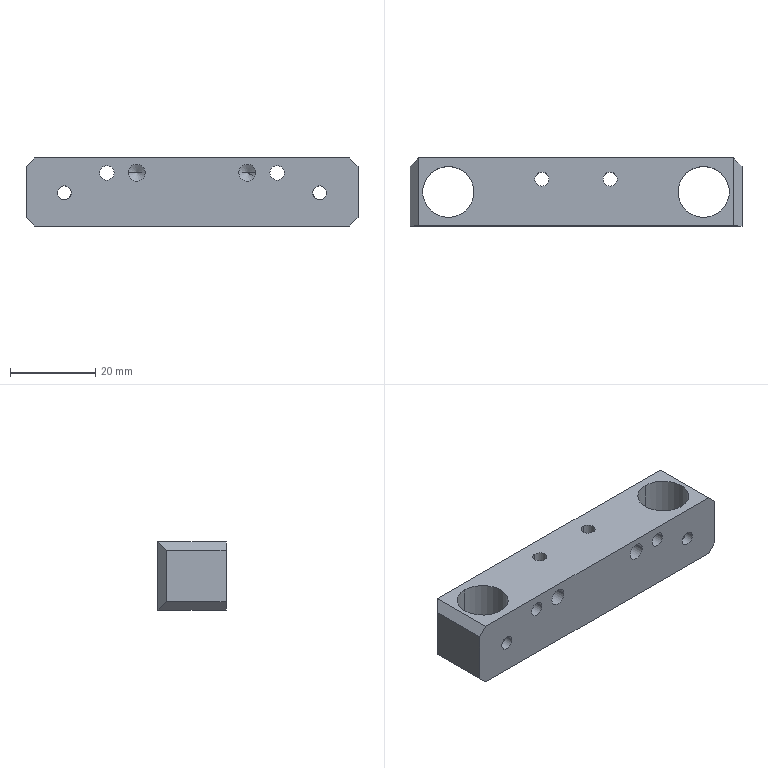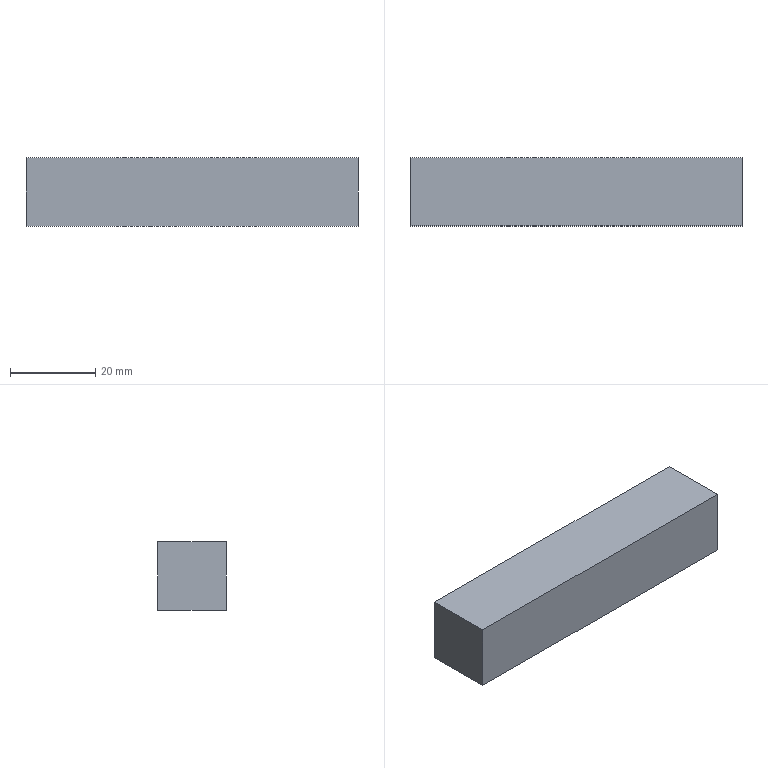CAM job | NX | 3+2 milling, drilling | part box 78 x 16 x 16 mm | stock box 78 x 16 x 16 mm
Tools:
number,name,description,diameter,corner_radius,flute_length,length,flutes
21,ZXZ,Milling Tool-5 Parameters,6.0,0.0,50.0,75.0,2
13,3.3ZT,Drilling Tool,3.3,0.0,35.0,50.0,2
24,3.4ZT,Drilling Tool,3.4,0.0,35.0,50.0,2
18,D2,Milling Tool-5 Parameters,2.0,0.0,50.0,75.0,2
1,D6A45,Milling Tool-5 Parameters,6.0,0.0,50.0,75.0,2
4,D10,Milling Tool-5 Parameters,10.0,0.0,50.0,75.0,2
17,D4,Milling Tool-5 Parameters,4.0,0.0,50.0,75.0,2
14,D10JING,Milling Tool-5 Parameters,10.0,0.0,50.0,75.0,2
Operations:
program,operation,operation_type,tool,method,geometry_group,spindle_rpm,surface_speed,feed_per_tooth,feed_cut,feed_plunge,cut_length_mm,path_length_mm,cut_time_min,machine_time_min
1,DRILLING,Operation,ZXZ,METHOD,A,3500.0,65.0,0.0357,250.0,0.0,24.0,187.303,0.096,0.1123
1,DRILLING_COPY_1,Operation,3.4ZT,METHOD,A,2000.0,21.0,0.0375,150.0,0.0,64.286,238.976,0.4286,0.446
1,DRILLING_COPY_1_COPY,Operation,3.3ZT,METHOD,A,2000.0,21.0,0.0375,150.0,0.0,41.983,207.041,0.2799,0.2964
1,HOLE_MILLING_2,CylinderMilling,D2,METHOD,A,7500.0,47.0,0.0533,800.0,100.0,5137.867,5302.867,6.422,6.439
1,ZLEVEL_PROFILE,ZLevelMilling,D10,METHOD,A,3500.0,109.0,0.3143,2200.0,1000.0,3430.847,3952.704,1.972,2.025
1,PLANAR_MILL,PlanarMilling,D6A45,METHOD,A,7500.0,141.0,0.0833,1250.0,100.0,258.996,727.126,0.2072,0.254
1,刀补18,CylinderMilling,D2,METHOD,A,7500.0,47.0,0.0533,800.0,100.0,149.518,314.518,0.1869,0.2034
2,HOLE_MILLING,CylinderMilling,D4,METHOD,B,5000.0,62.0,0.125,1250.0,100.0,631.51,797.31,0.5052,0.5218
2,PLANAR_MILL_COPY,PlanarMilling,D6A45,METHOD,B,7500.0,141.0,0.0833,1250.0,100.0,251.764,606.022,0.2014,0.2368
2,PLANAR_MILL_COPY_COPY,PlanarMilling,D6A45,METHOD,B,7500.0,141.0,0.0833,1250.0,100.0,173.963,848.412,0.1392,0.2066
3,DRILLING_COPY,Operation,ZXZ,METHOD,C,3500.0,65.0,0.0357,250.0,0.0,16.0,162.089,0.064,0.0786
3,DRILLING_COPY_1_COPY_COPY,Operation,3.3ZT,METHOD,C,2000.0,21.0,0.0375,150.0,0.0,41.983,163.244,0.2799,0.292
3,HOLE_MILLING_1,CylinderMilling,D10,METHOD,C,3500.0,0.0,0.0,2000.0,100.0,913.869,1124.869,0.4569,0.478
3,PLANAR_MILL_COPY_COPY_1,PlanarMilling,D6A45,METHOD,C,7500.0,141.0,0.0833,1250.0,100.0,291.806,652.661,0.2334,0.2695
3,刀补14,CylinderMilling,D10JING,METHOD,C,3500.0,0.0,0.0,2000.0,100.0,122.991,333.991,0.0615,0.0826